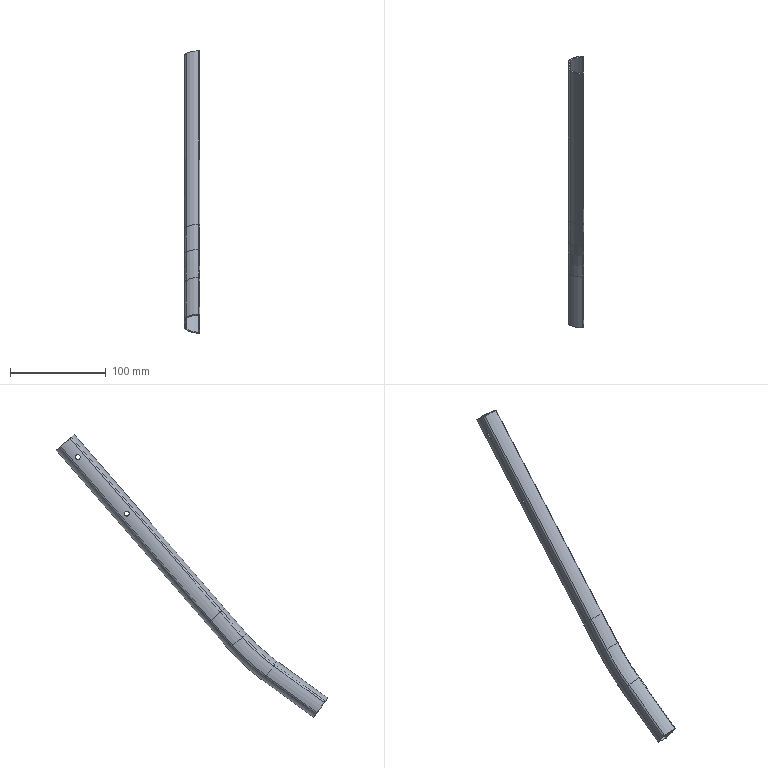Part | SolidWorks | features BaseBody 1 | 1 solid | 83 faces | box 16 x 283.583 x 295.302 mm | volume 30959 mm3 | cylinder 56 | spline 20 | plane 4 | torus 3 | commonest cylinder face diameters 5.2 x12 0.6 x8 3 x8 50 x6 3.6 x5 6 x5